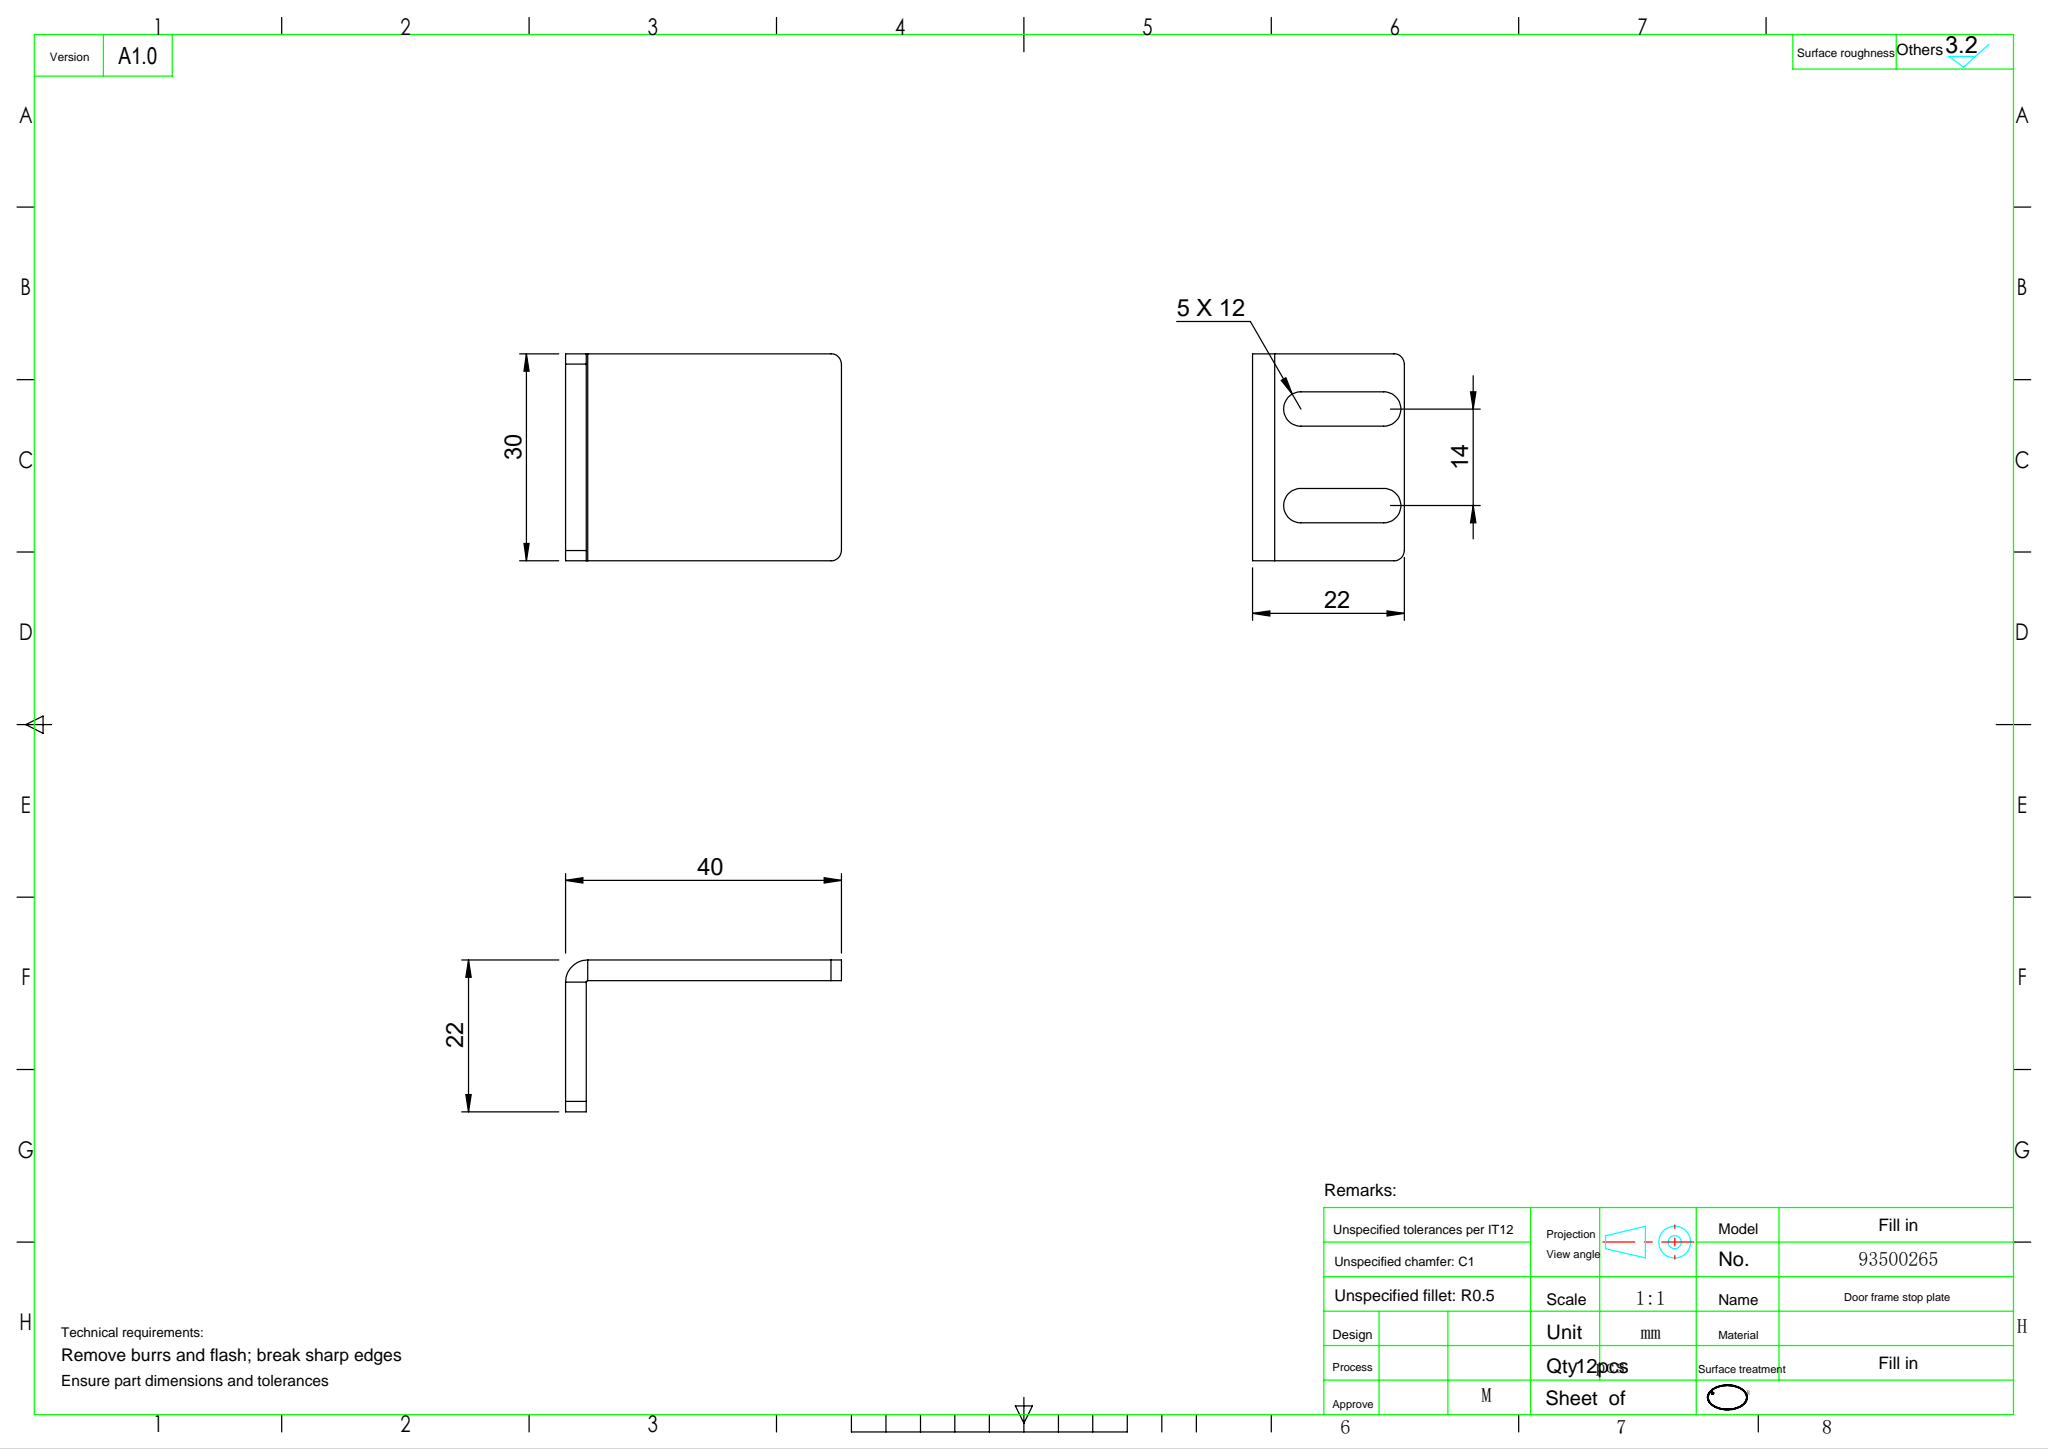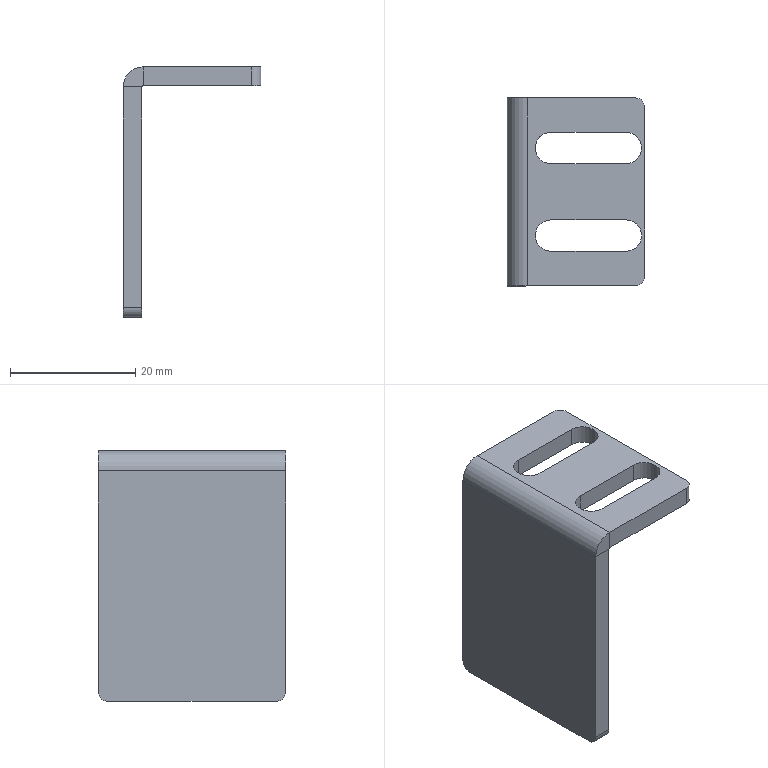Part | SolidWorks | features Fillet 1, FlatPattern 1, ICE 1, SMBaseFlange 1, SheetMetal 1 | 1 solid | 28 faces | box 22 x 30 x 40 mm | volume 4761 mm3 | plane 16 | cylinder 12 | commonest cylinder face diameters 5 x6 3 x4 0.4 x1 6.4 x1
STEP:
#1=CARTESIAN_POINT('',(4.5,8.,0.));
#2=VERTEX_POINT('',#1);
#3=CARTESIAN_POINT('',(7.,10.5,0.));
#4=VERTEX_POINT('',#3);
#5=CARTESIAN_POINT('',(7.,8.,0.));
#6=DIRECTION('',(0.,0.,-1.));
#7=DIRECTION('',(-1.,0.,0.));
#8=AXIS2_PLACEMENT_3D('',#5,#6,#7);
#9=CIRCLE('',#8,2.5);
#10=EDGE_CURVE('',#2,#4,#9,.T.);
#11=ORIENTED_EDGE('',*,*,#10,.F.);
#12=CARTESIAN_POINT('',(4.5,8.,-3.));
#13=VERTEX_POINT('',#12);
#14=CARTESIAN_POINT('',(4.5,8.,7.));
#15=DIRECTION('',(0.,0.,-1.));
#16=VECTOR('',#15,1000.);
#17=LINE('',#14,#16);
#18=EDGE_CURVE('',#2,#13,#17,.T.);
#19=ORIENTED_EDGE('',*,*,#18,.T.);
#20=CARTESIAN_POINT('',(7.,10.5,-3.));
#21=VERTEX_POINT('',#20);
#22=CARTESIAN_POINT('',(7.,8.,-3.));
#23=DIRECTION('',(0.,0.,-1.));
#24=DIRECTION('',(1.,0.,0.));
#25=AXIS2_PLACEMENT_3D('',#22,#23,#24);
#26=CIRCLE('',#25,2.5);
#27=EDGE_CURVE('',#13,#21,#26,.T.);
#28=ORIENTED_EDGE('',*,*,#27,.T.);
#29=CARTESIAN_POINT('',(7.,10.5,7.));
#30=DIRECTION('',(0.,0.,-1.));
#31=VECTOR('',#30,1000.);
#32=LINE('',#29,#31);
#33=EDGE_CURVE('',#4,#21,#32,.T.);
#34=ORIENTED_EDGE('',*,*,#33,.F.);
#35=EDGE_LOOP('',(#11,#19,#28,#34));
#36=FACE_OUTER_BOUND('',#35,.T.);
#37=CARTESIAN_POINT('',(7.,8.,7.));
#38=DIRECTION('',(0.,0.,-1.));
#39=DIRECTION('',(-1.,0.,0.));
#40=AXIS2_PLACEMENT_3D('',#37,#38,#39);
#41=CYLINDRICAL_SURFACE('',#40,2.5);
#42=ADVANCED_FACE('',(#36),#41,.F.);
#43=CARTESIAN_POINT('',(4.5,22.,0.));
#44=VERTEX_POINT('',#43);
#45=CARTESIAN_POINT('',(7.,24.5,0.));
#46=VERTEX_POINT('',#45);
#47=CARTESIAN_POINT('',(7.,22.,0.));
#48=DIRECTION('',(0.,0.,-1.));
#49=DIRECTION('',(-1.,0.,0.));
#50=AXIS2_PLACEMENT_3D('',#47,#48,#49);
#51=CIRCLE('',#50,2.5);
#52=EDGE_CURVE('',#44,#46,#51,.T.);
#53=ORIENTED_EDGE('',*,*,#52,.F.);
#54=CARTESIAN_POINT('',(4.5,22.,-3.));
#55=VERTEX_POINT('',#54);
#56=CARTESIAN_POINT('',(4.5,22.,7.));
#57=DIRECTION('',(0.,0.,-1.));
#58=VECTOR('',#57,1000.);
#59=LINE('',#56,#58);
#60=EDGE_CURVE('',#44,#55,#59,.T.);
#61=ORIENTED_EDGE('',*,*,#60,.T.);
#62=CARTESIAN_POINT('',(7.,24.5,-3.));
#63=VERTEX_POINT('',#62);
#64=CARTESIAN_POINT('',(7.,22.,-3.));
#65=DIRECTION('',(0.,0.,-1.));
#66=DIRECTION('',(-1.,0.,0.));
#67=AXIS2_PLACEMENT_3D('',#64,#65,#66);
#68=CIRCLE('',#67,2.5);
#69=EDGE_CURVE('',#55,#63,#68,.T.);
#70=ORIENTED_EDGE('',*,*,#69,.T.);
#71=CARTESIAN_POINT('',(7.,24.5,7.));
#72=DIRECTION('',(0.,0.,-1.));
#73=VECTOR('',#72,1000.);
#74=LINE('',#71,#73);
#75=EDGE_CURVE('',#46,#63,#74,.T.);
#76=ORIENTED_EDGE('',*,*,#75,.F.);
#77=EDGE_LOOP('',(#53,#61,#70,#76));
#78=FACE_OUTER_BOUND('',#77,.T.);
#79=CARTESIAN_POINT('',(7.,22.,7.));
#80=DIRECTION('',(0.,0.,-1.));
#81=DIRECTION('',(-1.,0.,0.));
#82=AXIS2_PLACEMENT_3D('',#79,#80,#81);
#83=CYLINDRICAL_SURFACE('',#82,2.5);
#84=ADVANCED_FACE('',(#78),#83,.F.);
#85=CARTESIAN_POINT('',(0.,30.,-3.2));
#86=VERTEX_POINT('',#85);
#87=CARTESIAN_POINT('',(3.,30.,-3.2));
#88=VERTEX_POINT('',#87);
#89=CARTESIAN_POINT('',(0.,30.,-3.2));
#90=DIRECTION('',(1.,0.,0.));
#91=VECTOR('',#90,1000.);
#92=LINE('',#89,#91);
#93=EDGE_CURVE('',#86,#88,#92,.T.);
#94=ORIENTED_EDGE('',*,*,#93,.F.);
#95=CARTESIAN_POINT('',(3.2,30.,0.));
#96=VERTEX_POINT('',#95);
#97=CARTESIAN_POINT('',(3.2,30.,-3.2));
#98=DIRECTION('',(0.,1.,0.));
#99=DIRECTION('',(0.,0.,-1.));
#100=AXIS2_PLACEMENT_3D('',#97,#98,#99);
#101=CIRCLE('',#100,3.2);
#102=EDGE_CURVE('',#86,#96,#101,.T.);
#103=ORIENTED_EDGE('',*,*,#102,.T.);
#104=CARTESIAN_POINT('',(3.2,30.,-3.));
#105=VERTEX_POINT('',#104);
#106=CARTESIAN_POINT('',(3.2,30.,-3.));
#107=DIRECTION('',(0.,0.,1.));
#108=VECTOR('',#107,1000.);
#109=LINE('',#106,#108);
#110=EDGE_CURVE('',#105,#96,#109,.T.);
#111=ORIENTED_EDGE('',*,*,#110,.F.);
#112=CARTESIAN_POINT('',(3.2,30.,-3.2));
#113=DIRECTION('',(0.,1.,0.));
#114=DIRECTION('',(1.,0.,0.));
#115=AXIS2_PLACEMENT_3D('',#112,#113,#114);
#116=CIRCLE('',#115,0.2);
#117=EDGE_CURVE('',#88,#105,#116,.T.);
#118=ORIENTED_EDGE('',*,*,#117,.F.);
#119=EDGE_LOOP('',(#94,#103,#111,#118));
#120=FACE_OUTER_BOUND('',#119,.T.);
#121=CARTESIAN_POINT('',(0.,30.,-3.2));
#122=DIRECTION('',(0.,1.,0.));
#123=DIRECTION('',(0.,0.,1.));
#124=AXIS2_PLACEMENT_3D('',#121,#122,#123);
#125=PLANE('',#124);
#126=ADVANCED_FACE('',(#120),#125,.T.);
#127=CARTESIAN_POINT('',(3.,30.,-38.5));
#128=VERTEX_POINT('',#127);
#129=CARTESIAN_POINT('',(3.,30.,-40.));
#130=DIRECTION('',(0.,0.,1.));
#131=VECTOR('',#130,1000.);
#132=LINE('',#129,#131);
#133=EDGE_CURVE('',#128,#88,#132,.T.);
#134=ORIENTED_EDGE('',*,*,#133,.F.);
#135=CARTESIAN_POINT('',(0.,30.,-38.5));
#136=VERTEX_POINT('',#135);
#137=CARTESIAN_POINT('',(3.2,30.,-38.5));
#138=DIRECTION('',(-1.,0.,0.));
#139=VECTOR('',#138,1000.);
#140=LINE('',#137,#139);
#141=EDGE_CURVE('',#128,#136,#140,.T.);
#142=ORIENTED_EDGE('',*,*,#141,.T.);
#143=CARTESIAN_POINT('',(0.,30.,-40.));
#144=DIRECTION('',(0.,0.,1.));
#145=VECTOR('',#144,1000.);
#146=LINE('',#143,#145);
#147=EDGE_CURVE('',#136,#86,#146,.T.);
#148=ORIENTED_EDGE('',*,*,#147,.T.);
#149=ORIENTED_EDGE('',*,*,#93,.T.);
#150=EDGE_LOOP('',(#134,#142,#148,#149));
#151=FACE_OUTER_BOUND('',#150,.T.);
#152=CARTESIAN_POINT('',(3.2,30.,-3.));
#153=DIRECTION('',(0.,1.,0.));
#154=DIRECTION('',(0.,0.,1.));
#155=AXIS2_PLACEMENT_3D('',#152,#153,#154);
#156=PLANE('',#155);
#157=ADVANCED_FACE('',(#151),#156,.T.);
#158=CARTESIAN_POINT('',(3.2,0.,0.));
#159=VERTEX_POINT('',#158);
#160=CARTESIAN_POINT('',(3.2,0.,-3.));
#161=VERTEX_POINT('',#160);
#162=CARTESIAN_POINT('',(3.2,0.,0.));
#163=DIRECTION('',(0.,0.,-1.));
#164=VECTOR('',#163,1000.);
#165=LINE('',#162,#164);
#166=EDGE_CURVE('',#159,#161,#165,.T.);
#167=ORIENTED_EDGE('',*,*,#166,.F.);
#168=CARTESIAN_POINT('',(0.,0.,-3.2));
#169=VERTEX_POINT('',#168);
#170=CARTESIAN_POINT('',(3.2,0.,-3.2));
#171=DIRECTION('',(0.,1.,0.));
#172=DIRECTION('',(0.,0.,-1.));
#173=AXIS2_PLACEMENT_3D('',#170,#171,#172);
#174=CIRCLE('',#173,3.2);
#175=EDGE_CURVE('',#169,#159,#174,.T.);
#176=ORIENTED_EDGE('',*,*,#175,.F.);
#177=CARTESIAN_POINT('',(3.,0.,-3.2));
#178=VERTEX_POINT('',#177);
#179=CARTESIAN_POINT('',(3.,0.,-3.2));
#180=DIRECTION('',(-1.,0.,0.));
#181=VECTOR('',#180,1000.);
#182=LINE('',#179,#181);
#183=EDGE_CURVE('',#178,#169,#182,.T.);
#184=ORIENTED_EDGE('',*,*,#183,.F.);
#185=CARTESIAN_POINT('',(3.2,0.,-3.2));
#186=DIRECTION('',(0.,1.,0.));
#187=DIRECTION('',(1.,0.,0.));
#188=AXIS2_PLACEMENT_3D('',#185,#186,#187);
#189=CIRCLE('',#188,0.2);
#190=EDGE_CURVE('',#178,#161,#189,.T.);
#191=ORIENTED_EDGE('',*,*,#190,.T.);
#192=EDGE_LOOP('',(#167,#176,#184,#191));
#193=FACE_OUTER_BOUND('',#192,.T.);
#194=CARTESIAN_POINT('',(3.2,0.,0.));
#195=DIRECTION('',(0.,-1.,0.));
#196=DIRECTION('',(0.,0.,-1.));
#197=AXIS2_PLACEMENT_3D('',#194,#195,#196);
#198=PLANE('',#197);
#199=ADVANCED_FACE('',(#193),#198,.T.);
#200=CARTESIAN_POINT('',(20.5,0.,-3.));
#201=VERTEX_POINT('',#200);
#202=CARTESIAN_POINT('',(0.,0.,-3.));
#203=DIRECTION('',(1.,0.,0.));
#204=VECTOR('',#203,1000.);
#205=LINE('',#202,#204);
#206=EDGE_CURVE('',#161,#201,#205,.T.);
#207=ORIENTED_EDGE('',*,*,#206,.T.);
#208=CARTESIAN_POINT('',(20.5,0.,0.));
#209=VERTEX_POINT('',#208);
#210=CARTESIAN_POINT('',(20.5,0.,-3.2));
#211=DIRECTION('',(0.,0.,1.));
#212=VECTOR('',#211,1000.);
#213=LINE('',#210,#212);
#214=EDGE_CURVE('',#201,#209,#213,.T.);
#215=ORIENTED_EDGE('',*,*,#214,.T.);
#216=CARTESIAN_POINT('',(0.,0.,0.));
#217=DIRECTION('',(1.,0.,0.));
#218=VECTOR('',#217,1000.);
#219=LINE('',#216,#218);
#220=EDGE_CURVE('',#159,#209,#219,.T.);
#221=ORIENTED_EDGE('',*,*,#220,.F.);
#222=ORIENTED_EDGE('',*,*,#166,.T.);
#223=EDGE_LOOP('',(#207,#215,#221,#222));
#224=FACE_OUTER_BOUND('',#223,.T.);
#225=CARTESIAN_POINT('',(3.,0.,-3.2));
#226=DIRECTION('',(0.,-1.,0.));
#227=DIRECTION('',(0.,0.,-1.));
#228=AXIS2_PLACEMENT_3D('',#225,#226,#227);
#229=PLANE('',#228);
#230=ADVANCED_FACE('',(#224),#229,.T.);
#231=CARTESIAN_POINT('',(19.,10.5,0.));
#232=VERTEX_POINT('',#231);
#233=CARTESIAN_POINT('',(0.,10.5,0.));
#234=DIRECTION('',(1.,0.,0.));
#235=VECTOR('',#234,1000.);
#236=LINE('',#233,#235);
#237=EDGE_CURVE('',#4,#232,#236,.T.);
#238=ORIENTED_EDGE('',*,*,#237,.T.);
#239=CARTESIAN_POINT('',(19.,5.5,0.));
#240=VERTEX_POINT('',#239);
#241=CARTESIAN_POINT('',(19.,8.,0.));
#242=DIRECTION('',(0.,0.,-1.));
#243=DIRECTION('',(-1.,0.,0.));
#244=AXIS2_PLACEMENT_3D('',#241,#242,#243);
#245=CIRCLE('',#244,2.5);
#246=EDGE_CURVE('',#232,#240,#245,.T.);
#247=ORIENTED_EDGE('',*,*,#246,.T.);
#248=CARTESIAN_POINT('',(7.,5.5,0.));
#249=VERTEX_POINT('',#248);
#250=CARTESIAN_POINT('',(0.,5.5,0.));
#251=DIRECTION('',(-1.,0.,0.));
#252=VECTOR('',#251,1000.);
#253=LINE('',#250,#252);
#254=EDGE_CURVE('',#240,#249,#253,.T.);
#255=ORIENTED_EDGE('',*,*,#254,.T.);
#256=CARTESIAN_POINT('',(7.,8.,0.));
#257=DIRECTION('',(0.,0.,-1.));
#258=DIRECTION('',(-1.,0.,0.));
#259=AXIS2_PLACEMENT_3D('',#256,#257,#258);
#260=CIRCLE('',#259,2.5);
#261=EDGE_CURVE('',#249,#2,#260,.T.);
#262=ORIENTED_EDGE('',*,*,#261,.T.);
#263=ORIENTED_EDGE('',*,*,#10,.T.);
#264=EDGE_LOOP('',(#238,#247,#255,#262,#263));
#265=FACE_BOUND('',#264,.T.);
#266=CARTESIAN_POINT('',(19.,24.5,0.));
#267=VERTEX_POINT('',#266);
#268=CARTESIAN_POINT('',(0.,24.5,0.));
#269=DIRECTION('',(1.,0.,0.));
#270=VECTOR('',#269,1000.);
#271=LINE('',#268,#270);
#272=EDGE_CURVE('',#46,#267,#271,.T.);
#273=ORIENTED_EDGE('',*,*,#272,.T.);
#274=CARTESIAN_POINT('',(19.,19.5,0.));
#275=VERTEX_POINT('',#274);
#276=CARTESIAN_POINT('',(19.,22.,0.));
#277=DIRECTION('',(0.,0.,-1.));
#278=DIRECTION('',(-1.,0.,0.));
#279=AXIS2_PLACEMENT_3D('',#276,#277,#278);
#280=CIRCLE('',#279,2.5);
#281=EDGE_CURVE('',#267,#275,#280,.T.);
#282=ORIENTED_EDGE('',*,*,#281,.T.);
#283=CARTESIAN_POINT('',(7.,19.5,0.));
#284=VERTEX_POINT('',#283);
#285=CARTESIAN_POINT('',(0.,19.5,0.));
#286=DIRECTION('',(-1.,0.,0.));
#287=VECTOR('',#286,1000.);
#288=LINE('',#285,#287);
#289=EDGE_CURVE('',#275,#284,#288,.T.);
#290=ORIENTED_EDGE('',*,*,#289,.T.);
#291=CARTESIAN_POINT('',(7.,22.,0.));
#292=DIRECTION('',(0.,0.,-1.));
#293=DIRECTION('',(-1.,0.,0.));
#294=AXIS2_PLACEMENT_3D('',#291,#292,#293);
#295=CIRCLE('',#294,2.5);
#296=EDGE_CURVE('',#284,#44,#295,.T.);
#297=ORIENTED_EDGE('',*,*,#296,.T.);
#298=ORIENTED_EDGE('',*,*,#52,.T.);
#299=EDGE_LOOP('',(#273,#282,#290,#297,#298));
#300=FACE_BOUND('',#299,.T.);
#301=CARTESIAN_POINT('',(22.,28.5,0.));
#302=VERTEX_POINT('',#301);
#303=CARTESIAN_POINT('',(22.,1.5,0.));
#304=VERTEX_POINT('',#303);
#305=CARTESIAN_POINT('',(22.,30.,0.));
#306=DIRECTION('',(0.,-1.,0.));
#307=VECTOR('',#306,1000.);
#308=LINE('',#305,#307);
#309=EDGE_CURVE('',#302,#304,#308,.T.);
#310=ORIENTED_EDGE('',*,*,#309,.F.);
#311=CARTESIAN_POINT('',(20.5,30.,0.));
#312=VERTEX_POINT('',#311);
#313=CARTESIAN_POINT('',(20.5,28.5,0.));
#314=DIRECTION('',(0.,0.,1.));
#315=DIRECTION('',(-1.,0.,0.));
#316=AXIS2_PLACEMENT_3D('',#313,#314,#315);
#317=CIRCLE('',#316,1.5);
#318=EDGE_CURVE('',#302,#312,#317,.T.);
#319=ORIENTED_EDGE('',*,*,#318,.T.);
#320=CARTESIAN_POINT('',(0.,30.,0.));
#321=DIRECTION('',(1.,0.,0.));
#322=VECTOR('',#321,1000.);
#323=LINE('',#320,#322);
#324=EDGE_CURVE('',#96,#312,#323,.T.);
#325=ORIENTED_EDGE('',*,*,#324,.F.);
#326=CARTESIAN_POINT('',(3.2,30.,0.));
#327=DIRECTION('',(0.,-1.,0.));
#328=VECTOR('',#327,1000.);
#329=LINE('',#326,#328);
#330=EDGE_CURVE('',#96,#159,#329,.T.);
#331=ORIENTED_EDGE('',*,*,#330,.T.);
#332=ORIENTED_EDGE('',*,*,#220,.T.);
#333=CARTESIAN_POINT('',(20.5,1.5,0.));
#334=DIRECTION('',(0.,0.,1.));
#335=DIRECTION('',(-1.,0.,0.));
#336=AXIS2_PLACEMENT_3D('',#333,#334,#335);
#337=CIRCLE('',#336,1.5);
#338=EDGE_CURVE('',#209,#304,#337,.T.);
#339=ORIENTED_EDGE('',*,*,#338,.T.);
#340=EDGE_LOOP('',(#310,#319,#325,#331,#332,#339));
#341=FACE_OUTER_BOUND('',#340,.T.);
#342=CARTESIAN_POINT('',(0.,30.,0.));
#343=DIRECTION('',(0.,0.,-1.));
#344=DIRECTION('',(-1.,0.,0.));
#345=AXIS2_PLACEMENT_3D('',#342,#343,#344);
#346=PLANE('',#345);
#347=ADVANCED_FACE('',(#265,#300,#341),#346,.F.);
#348=CARTESIAN_POINT('',(22.,28.5,-3.));
#349=VERTEX_POINT('',#348);
#350=CARTESIAN_POINT('',(22.,1.5,-3.));
#351=VERTEX_POINT('',#350);
#352=CARTESIAN_POINT('',(22.,30.,-3.));
#353=DIRECTION('',(0.,-1.,0.));
#354=VECTOR('',#353,1000.);
#355=LINE('',#352,#354);
#356=EDGE_CURVE('',#349,#351,#355,.T.);
#357=ORIENTED_EDGE('',*,*,#356,.F.);
#358=CARTESIAN_POINT('',(22.,28.5,-3.));
#359=DIRECTION('',(0.,0.,1.));
#360=VECTOR('',#359,1000.);
#361=LINE('',#358,#360);
#362=EDGE_CURVE('',#349,#302,#361,.T.);
#363=ORIENTED_EDGE('',*,*,#362,.T.);
#364=ORIENTED_EDGE('',*,*,#309,.T.);
#365=CARTESIAN_POINT('',(22.,1.5,-3.));
#366=DIRECTION('',(0.,0.,-1.));
#367=VECTOR('',#366,1000.);
#368=LINE('',#365,#367);
#369=EDGE_CURVE('',#304,#351,#368,.T.);
#370=ORIENTED_EDGE('',*,*,#369,.T.);
#371=EDGE_LOOP('',(#357,#363,#364,#370));
#372=FACE_OUTER_BOUND('',#371,.T.);
#373=CARTESIAN_POINT('',(22.,30.,-3.));
#374=DIRECTION('',(1.,0.,0.));
#375=DIRECTION('',(0.,0.,-1.));
#376=AXIS2_PLACEMENT_3D('',#373,#374,#375);
#377=PLANE('',#376);
#378=ADVANCED_FACE('',(#372),#377,.T.);
#379=CARTESIAN_POINT('',(19.,10.5,-3.));
#380=VERTEX_POINT('',#379);
#381=CARTESIAN_POINT('',(19.,5.5,-3.));
#382=VERTEX_POINT('',#381);
#383=CARTESIAN_POINT('',(19.,8.,-3.));
#384=DIRECTION('',(0.,0.,-1.));
#385=DIRECTION('',(1.,0.,0.));
#386=AXIS2_PLACEMENT_3D('',#383,#384,#385);
#387=CIRCLE('',#386,2.5);
#388=EDGE_CURVE('',#380,#382,#387,.T.);
#389=ORIENTED_EDGE('',*,*,#388,.F.);
#390=CARTESIAN_POINT('',(19.,10.5,-3.));
#391=DIRECTION('',(1.,0.,0.));
#392=VECTOR('',#391,1000.);
#393=LINE('',#390,#392);
#394=EDGE_CURVE('',#21,#380,#393,.T.);
#395=ORIENTED_EDGE('',*,*,#394,.F.);
#396=ORIENTED_EDGE('',*,*,#27,.F.);
#397=CARTESIAN_POINT('',(7.,5.5,-3.));
#398=VERTEX_POINT('',#397);
#399=CARTESIAN_POINT('',(7.,8.,-3.));
#400=DIRECTION('',(0.,0.,-1.));
#401=DIRECTION('',(1.,0.,0.));
#402=AXIS2_PLACEMENT_3D('',#399,#400,#401);
#403=CIRCLE('',#402,2.5);
#404=EDGE_CURVE('',#398,#13,#403,.T.);
#405=ORIENTED_EDGE('',*,*,#404,.F.);
#406=CARTESIAN_POINT('',(19.,5.5,-3.));
#407=DIRECTION('',(-1.,0.,0.));
#408=VECTOR('',#407,1000.);
#409=LINE('',#406,#408);
#410=EDGE_CURVE('',#382,#398,#409,.T.);
#411=ORIENTED_EDGE('',*,*,#410,.F.);
#412=EDGE_LOOP('',(#389,#395,#396,#405,#411));
#413=FACE_BOUND('',#412,.T.);
#414=CARTESIAN_POINT('',(19.,24.5,-3.));
#415=VERTEX_POINT('',#414);
#416=CARTESIAN_POINT('',(19.,19.5,-3.));
#417=VERTEX_POINT('',#416);
#418=CARTESIAN_POINT('',(19.,22.,-3.));
#419=DIRECTION('',(0.,0.,-1.));
#420=DIRECTION('',(-1.,0.,0.));
#421=AXIS2_PLACEMENT_3D('',#418,#419,#420);
#422=CIRCLE('',#421,2.5);
#423=EDGE_CURVE('',#415,#417,#422,.T.);
#424=ORIENTED_EDGE('',*,*,#423,.F.);
#425=CARTESIAN_POINT('',(19.,24.5,-3.));
#426=DIRECTION('',(1.,0.,0.));
#427=VECTOR('',#426,1000.);
#428=LINE('',#425,#427);
#429=EDGE_CURVE('',#63,#415,#428,.T.);
#430=ORIENTED_EDGE('',*,*,#429,.F.);
#431=ORIENTED_EDGE('',*,*,#69,.F.);
#432=CARTESIAN_POINT('',(7.,19.5,-3.));
#433=VERTEX_POINT('',#432);
#434=CARTESIAN_POINT('',(7.,22.,-3.));
#435=DIRECTION('',(0.,0.,-1.));
#436=DIRECTION('',(-1.,0.,0.));
#437=AXIS2_PLACEMENT_3D('',#434,#435,#436);
#438=CIRCLE('',#437,2.5);
#439=EDGE_CURVE('',#433,#55,#438,.T.);
#440=ORIENTED_EDGE('',*,*,#439,.F.);
#441=CARTESIAN_POINT('',(19.,19.5,-3.));
#442=DIRECTION('',(-1.,0.,0.));
#443=VECTOR('',#442,1000.);
#444=LINE('',#441,#443);
#445=EDGE_CURVE('',#417,#433,#444,.T.);
#446=ORIENTED_EDGE('',*,*,#445,.F.);
#447=EDGE_LOOP('',(#424,#430,#431,#440,#446));
#448=FACE_BOUND('',#447,.T.);
#449=CARTESIAN_POINT('',(20.5,30.,-3.));
#450=VERTEX_POINT('',#449);
#451=CARTESIAN_POINT('',(0.,30.,-3.));
#452=DIRECTION('',(1.,0.,0.));
#453=VECTOR('',#452,1000.);
#454=LINE('',#451,#453);
#455=EDGE_CURVE('',#105,#450,#454,.T.);
#456=ORIENTED_EDGE('',*,*,#455,.T.);
#457=CARTESIAN_POINT('',(20.5,28.5,-3.));
#458=DIRECTION('',(0.,0.,-1.));
#459=DIRECTION('',(-1.,0.,0.));
#460=AXIS2_PLACEMENT_3D('',#457,#458,#459);
#461=CIRCLE('',#460,1.5);
#462=EDGE_CURVE('',#450,#349,#461,.T.);
#463=ORIENTED_EDGE('',*,*,#462,.T.);
#464=ORIENTED_EDGE('',*,*,#356,.T.);
#465=CARTESIAN_POINT('',(20.5,1.5,-3.));
#466=DIRECTION('',(0.,0.,-1.));
#467=DIRECTION('',(-1.,0.,0.));
#468=AXIS2_PLACEMENT_3D('',#465,#466,#467);
#469=CIRCLE('',#468,1.5);
#470=EDGE_CURVE('',#351,#201,#469,.T.);
#471=ORIENTED_EDGE('',*,*,#470,.T.);
#472=ORIENTED_EDGE('',*,*,#206,.F.);
#473=CARTESIAN_POINT('',(3.2,30.,-3.));
#474=DIRECTION('',(0.,-1.,0.));
#475=VECTOR('',#474,1000.);
#476=LINE('',#473,#475);
#477=EDGE_CURVE('',#105,#161,#476,.T.);
#478=ORIENTED_EDGE('',*,*,#477,.F.);
#479=EDGE_LOOP('',(#456,#463,#464,#471,#472,#478));
#480=FACE_OUTER_BOUND('',#479,.T.);
#481=CARTESIAN_POINT('',(0.,30.,-3.));
#482=DIRECTION('',(0.,0.,-1.));
#483=DIRECTION('',(-1.,0.,0.));
#484=AXIS2_PLACEMENT_3D('',#481,#482,#483);
#485=PLANE('',#484);
#486=ADVANCED_FACE('',(#413,#448,#480),#485,.T.);
#487=ORIENTED_EDGE('',*,*,#190,.F.);
#488=CARTESIAN_POINT('',(3.,30.,-3.2));
#489=DIRECTION('',(0.,-1.,0.));
#490=VECTOR('',#489,1000.);
#491=LINE('',#488,#490);
#492=EDGE_CURVE('',#88,#178,#491,.T.);
#493=ORIENTED_EDGE('',*,*,#492,.F.);
#494=ORIENTED_EDGE('',*,*,#117,.T.);
#495=ORIENTED_EDGE('',*,*,#477,.T.);
#496=EDGE_LOOP('',(#487,#493,#494,#495));
#497=FACE_OUTER_BOUND('',#496,.T.);
#498=CARTESIAN_POINT('',(3.2,30.,-3.2));
#499=DIRECTION('',(0.,-1.,0.));
#500=DIRECTION('',(0.,0.,-1.));
#501=AXIS2_PLACEMENT_3D('',#498,#499,#500);
#502=CYLINDRICAL_SURFACE('',#501,0.2);
#503=ADVANCED_FACE('',(#497),#502,.F.);
#504=CARTESIAN_POINT('',(3.,28.5,-40.));
#505=VERTEX_POINT('',#504);
#506=CARTESIAN_POINT('',(3.,1.5,-40.));
#507=VERTEX_POINT('',#506);
#508=CARTESIAN_POINT('',(3.,30.,-40.));
#509=DIRECTION('',(0.,-1.,0.));
#510=VECTOR('',#509,1000.);
#511=LINE('',#508,#510);
#512=EDGE_CURVE('',#505,#507,#511,.T.);
#513=ORIENTED_EDGE('',*,*,#512,.F.);
#514=CARTESIAN_POINT('',(3.,28.5,-38.5));
#515=DIRECTION('',(1.,0.,0.));
#516=DIRECTION('',(0.,0.,-1.));
#517=AXIS2_PLACEMENT_3D('',#514,#515,#516);
#518=CIRCLE('',#517,1.5);
#519=EDGE_CURVE('',#505,#128,#518,.T.);
#520=ORIENTED_EDGE('',*,*,#519,.T.);
#521=ORIENTED_EDGE('',*,*,#133,.T.);
#522=ORIENTED_EDGE('',*,*,#492,.T.);
#523=CARTESIAN_POINT('',(3.,0.,-38.5));
#524=VERTEX_POINT('',#523);
#525=CARTESIAN_POINT('',(3.,0.,-40.));
#526=DIRECTION('',(0.,0.,1.));
#527=VECTOR('',#526,1000.);
#528=LINE('',#525,#527);
#529=EDGE_CURVE('',#524,#178,#528,.T.);
#530=ORIENTED_EDGE('',*,*,#529,.F.);
#531=CARTESIAN_POINT('',(3.,1.5,-38.5));
#532=DIRECTION('',(1.,0.,0.));
#533=DIRECTION('',(0.,0.,-1.));
#534=AXIS2_PLACEMENT_3D('',#531,#532,#533);
#535=CIRCLE('',#534,1.5);
#536=EDGE_CURVE('',#524,#507,#535,.T.);
#537=ORIENTED_EDGE('',*,*,#536,.T.);
#538=EDGE_LOOP('',(#513,#520,#521,#522,#530,#537));
#539=FACE_OUTER_BOUND('',#538,.T.);
#540=CARTESIAN_POINT('',(3.,30.,-40.));
#541=DIRECTION('',(1.,0.,0.));
#542=DIRECTION('',(0.,0.,-1.));
#543=AXIS2_PLACEMENT_3D('',#540,#541,#542);
#544=PLANE('',#543);
#545=ADVANCED_FACE('',(#539),#544,.T.);
#546=CARTESIAN_POINT('',(0.,28.5,-40.));
#547=VERTEX_POINT('',#546);
#548=CARTESIAN_POINT('',(0.,1.5,-40.));
#549=VERTEX_POINT('',#548);
#550=CARTESIAN_POINT('',(0.,30.,-40.));
#551=DIRECTION('',(0.,-1.,0.));
#552=VECTOR('',#551,1000.);
#553=LINE('',#550,#552);
#554=EDGE_CURVE('',#547,#549,#553,.T.);
#555=ORIENTED_EDGE('',*,*,#554,.F.);
#556=CARTESIAN_POINT('',(0.,28.5,-40.));
#557=DIRECTION('',(1.,0.,0.));
#558=VECTOR('',#557,1000.);
#559=LINE('',#556,#558);
#560=EDGE_CURVE('',#547,#505,#559,.T.);
#561=ORIENTED_EDGE('',*,*,#560,.T.);
#562=ORIENTED_EDGE('',*,*,#512,.T.);
#563=CARTESIAN_POINT('',(0.,1.5,-40.));
#564=DIRECTION('',(-1.,0.,0.));
#565=VECTOR('',#564,1000.);
#566=LINE('',#563,#565);
#567=EDGE_CURVE('',#507,#549,#566,.T.);
#568=ORIENTED_EDGE('',*,*,#567,.T.);
#569=EDGE_LOOP('',(#555,#561,#562,#568));
#570=FACE_OUTER_BOUND('',#569,.T.);
#571=CARTESIAN_POINT('',(0.,30.,-40.));
#572=DIRECTION('',(0.,0.,-1.));
#573=DIRECTION('',(-1.,0.,0.));
#574=AXIS2_PLACEMENT_3D('',#571,#572,#573);
#575=PLANE('',#574);
#576=ADVANCED_FACE('',(#570),#575,.T.);
#577=ORIENTED_EDGE('',*,*,#147,.F.);
#578=CARTESIAN_POINT('',(0.,28.5,-38.5));
#579=DIRECTION('',(-1.,0.,0.));
#580=DIRECTION('',(0.,0.,-1.));
#581=AXIS2_PLACEMENT_3D('',#578,#579,#580);
#582=CIRCLE('',#581,1.5);
#583=EDGE_CURVE('',#136,#547,#582,.T.);
#584=ORIENTED_EDGE('',*,*,#583,.T.);
#585=ORIENTED_EDGE('',*,*,#554,.T.);
#586=CARTESIAN_POINT('',(0.,0.,-38.5));
#587=VERTEX_POINT('',#586);
#588=CARTESIAN_POINT('',(0.,1.5,-38.5));
#589=DIRECTION('',(-1.,0.,0.));
#590=DIRECTION('',(0.,0.,-1.));
#591=AXIS2_PLACEMENT_3D('',#588,#589,#590);
#592=CIRCLE('',#591,1.5);
#593=EDGE_CURVE('',#549,#587,#592,.T.);
#594=ORIENTED_EDGE('',*,*,#593,.T.);
#595=CARTESIAN_POINT('',(0.,0.,-40.));
#596=DIRECTION('',(0.,0.,1.));
#597=VECTOR('',#596,1000.);
#598=LINE('',#595,#597);
#599=EDGE_CURVE('',#587,#169,#598,.T.);
#600=ORIENTED_EDGE('',*,*,#599,.T.);
#601=CARTESIAN_POINT('',(0.,30.,-3.2));
#602=DIRECTION('',(0.,-1.,0.));
#603=VECTOR('',#602,1000.);
#604=LINE('',#601,#603);
#605=EDGE_CURVE('',#86,#169,#604,.T.);
#606=ORIENTED_EDGE('',*,*,#605,.F.);
#607=EDGE_LOOP('',(#577,#584,#585,#594,#600,#606));
#608=FACE_OUTER_BOUND('',#607,.T.);
#609=CARTESIAN_POINT('',(0.,30.,-40.));
#610=DIRECTION('',(1.,0.,0.));
#611=DIRECTION('',(0.,0.,-1.));
#612=AXIS2_PLACEMENT_3D('',#609,#610,#611);
#613=PLANE('',#612);
#614=ADVANCED_FACE('',(#608),#613,.F.);
#615=ORIENTED_EDGE('',*,*,#175,.T.);
#616=ORIENTED_EDGE('',*,*,#330,.F.);
#617=ORIENTED_EDGE('',*,*,#102,.F.);
#618=ORIENTED_EDGE('',*,*,#605,.T.);
#619=EDGE_LOOP('',(#615,#616,#617,#618));
#620=FACE_OUTER_BOUND('',#619,.T.);
#621=CARTESIAN_POINT('',(3.2,30.,-3.2));
#622=DIRECTION('',(0.,-1.,0.));
#623=DIRECTION('',(0.,0.,-1.));
#624=AXIS2_PLACEMENT_3D('',#621,#622,#623);
#625=CYLINDRICAL_SURFACE('',#624,3.2);
#626=ADVANCED_FACE('',(#620),#625,.T.);
#627=ORIENTED_EDGE('',*,*,#324,.T.);
#628=CARTESIAN_POINT('',(20.5,30.,-3.2));
#629=DIRECTION('',(0.,0.,-1.));
#630=VECTOR('',#629,1000.);
#631=LINE('',#628,#630);
#632=EDGE_CURVE('',#312,#450,#631,.T.);
#633=ORIENTED_EDGE('',*,*,#632,.T.);
#634=ORIENTED_EDGE('',*,*,#455,.F.);
#635=ORIENTED_EDGE('',*,*,#110,.T.);
#636=EDGE_LOOP('',(#627,#633,#634,#635));
#637=FACE_OUTER_BOUND('',#636,.T.);
#638=CARTESIAN_POINT('',(3.2,30.,-3.2));
#639=DIRECTION('',(0.,1.,0.));
#640=DIRECTION('',(1.,0.,0.));
#641=AXIS2_PLACEMENT_3D('',#638,#639,#640);
#642=PLANE('',#641);
#643=ADVANCED_FACE('',(#637),#642,.T.);
#644=ORIENTED_EDGE('',*,*,#599,.F.);
#645=CARTESIAN_POINT('',(3.,0.,-38.5));
#646=DIRECTION('',(1.,0.,0.));
#647=VECTOR('',#646,1000.);
#648=LINE('',#645,#647);
#649=EDGE_CURVE('',#587,#524,#648,.T.);
#650=ORIENTED_EDGE('',*,*,#649,.T.);
#651=ORIENTED_EDGE('',*,*,#529,.T.);
#652=ORIENTED_EDGE('',*,*,#183,.T.);
#653=EDGE_LOOP('',(#644,#650,#651,#652));
#654=FACE_OUTER_BOUND('',#653,.T.);
#655=CARTESIAN_POINT('',(3.2,0.,-3.2));
#656=DIRECTION('',(0.,1.,0.));
#657=DIRECTION('',(1.,0.,0.));
#658=AXIS2_PLACEMENT_3D('',#655,#656,#657);
#659=PLANE('',#658);
#660=ADVANCED_FACE('',(#654),#659,.F.);
#661=ORIENTED_EDGE('',*,*,#583,.F.);
#662=ORIENTED_EDGE('',*,*,#141,.F.);
#663=ORIENTED_EDGE('',*,*,#519,.F.);
#664=ORIENTED_EDGE('',*,*,#560,.F.);
#665=EDGE_LOOP('',(#661,#662,#663,#664));
#666=FACE_OUTER_BOUND('',#665,.T.);
#667=CARTESIAN_POINT('',(0.,28.5,-38.5));
#668=DIRECTION('',(1.,0.,0.));
#669=DIRECTION('',(0.,0.,-1.));
#670=AXIS2_PLACEMENT_3D('',#667,#668,#669);
#671=CYLINDRICAL_SURFACE('',#670,1.5);
#672=ADVANCED_FACE('',(#666),#671,.T.);
#673=ORIENTED_EDGE('',*,*,#593,.F.);
#674=ORIENTED_EDGE('',*,*,#567,.F.);
#675=ORIENTED_EDGE('',*,*,#536,.F.);
#676=ORIENTED_EDGE('',*,*,#649,.F.);
#677=EDGE_LOOP('',(#673,#674,#675,#676));
#678=FACE_OUTER_BOUND('',#677,.T.);
#679=CARTESIAN_POINT('',(3.2,1.5,-38.5));
#680=DIRECTION('',(-1.,0.,0.));
#681=DIRECTION('',(0.,0.,1.));
#682=AXIS2_PLACEMENT_3D('',#679,#680,#681);
#683=CYLINDRICAL_SURFACE('',#682,1.5);
#684=ADVANCED_FACE('',(#678),#683,.T.);
#685=ORIENTED_EDGE('',*,*,#462,.F.);
#686=ORIENTED_EDGE('',*,*,#632,.F.);
#687=ORIENTED_EDGE('',*,*,#318,.F.);
#688=ORIENTED_EDGE('',*,*,#362,.F.);
#689=EDGE_LOOP('',(#685,#686,#687,#688));
#690=FACE_OUTER_BOUND('',#689,.T.);
#691=CARTESIAN_POINT('',(20.5,28.5,-3.));
#692=DIRECTION('',(0.,0.,1.));
#693=DIRECTION('',(1.,0.,0.));
#694=AXIS2_PLACEMENT_3D('',#691,#692,#693);
#695=CYLINDRICAL_SURFACE('',#694,1.5);
#696=ADVANCED_FACE('',(#690),#695,.T.);
#697=ORIENTED_EDGE('',*,*,#470,.F.);
#698=ORIENTED_EDGE('',*,*,#369,.F.);
#699=ORIENTED_EDGE('',*,*,#338,.F.);
#700=ORIENTED_EDGE('',*,*,#214,.F.);
#701=EDGE_LOOP('',(#697,#698,#699,#700));
#702=FACE_OUTER_BOUND('',#701,.T.);
#703=CARTESIAN_POINT('',(20.5,1.5,-3.2));
#704=DIRECTION('',(0.,0.,1.));
#705=DIRECTION('',(1.,0.,0.));
#706=AXIS2_PLACEMENT_3D('',#703,#704,#705);
#707=CYLINDRICAL_SURFACE('',#706,1.5);
#708=ADVANCED_FACE('',(#702),#707,.T.);
#709=CARTESIAN_POINT('',(19.,24.5,7.));
#710=DIRECTION('',(0.,0.,-1.));
#711=VECTOR('',#710,1000.);
#712=LINE('',#709,#711);
#713=EDGE_CURVE('',#267,#415,#712,.T.);
#714=ORIENTED_EDGE('',*,*,#713,.T.);
#715=ORIENTED_EDGE('',*,*,#423,.T.);
#716=CARTESIAN_POINT('',(19.,19.5,7.));
#717=DIRECTION('',(0.,0.,-1.));
#718=VECTOR('',#717,1000.);
#719=LINE('',#716,#718);
#720=EDGE_CURVE('',#275,#417,#719,.T.);
#721=ORIENTED_EDGE('',*,*,#720,.F.);
#722=ORIENTED_EDGE('',*,*,#281,.F.);
#723=EDGE_LOOP('',(#714,#715,#721,#722));
#724=FACE_OUTER_BOUND('',#723,.T.);
#725=CARTESIAN_POINT('',(19.,22.,7.));
#726=DIRECTION('',(0.,0.,-1.));
#727=DIRECTION('',(-1.,0.,0.));
#728=AXIS2_PLACEMENT_3D('',#725,#726,#727);
#729=CYLINDRICAL_SURFACE('',#728,2.5);
#730=ADVANCED_FACE('',(#724),#729,.F.);
#731=ORIENTED_EDGE('',*,*,#75,.T.);
#732=ORIENTED_EDGE('',*,*,#429,.T.);
#733=ORIENTED_EDGE('',*,*,#713,.F.);
#734=ORIENTED_EDGE('',*,*,#272,.F.);
#735=EDGE_LOOP('',(#731,#732,#733,#734));
#736=FACE_OUTER_BOUND('',#735,.T.);
#737=CARTESIAN_POINT('',(19.,24.5,7.));
#738=DIRECTION('',(0.,1.,0.));
#739=DIRECTION('',(0.,0.,1.));
#740=AXIS2_PLACEMENT_3D('',#737,#738,#739);
#741=PLANE('',#740);
#742=ADVANCED_FACE('',(#736),#741,.F.);
#743=ORIENTED_EDGE('',*,*,#60,.F.);
#744=ORIENTED_EDGE('',*,*,#296,.F.);
#745=CARTESIAN_POINT('',(7.,19.5,7.));
#746=DIRECTION('',(0.,0.,-1.));
#747=VECTOR('',#746,1000.);
#748=LINE('',#745,#747);
#749=EDGE_CURVE('',#284,#433,#748,.T.);
#750=ORIENTED_EDGE('',*,*,#749,.T.);
#751=ORIENTED_EDGE('',*,*,#439,.T.);
#752=EDGE_LOOP('',(#743,#744,#750,#751));
#753=FACE_OUTER_BOUND('',#752,.T.);
#754=CARTESIAN_POINT('',(7.,22.,7.));
#755=DIRECTION('',(0.,0.,-1.));
#756=DIRECTION('',(-1.,0.,0.));
#757=AXIS2_PLACEMENT_3D('',#754,#755,#756);
#758=CYLINDRICAL_SURFACE('',#757,2.5);
#759=ADVANCED_FACE('',(#753),#758,.F.);
#760=ORIENTED_EDGE('',*,*,#720,.T.);
#761=ORIENTED_EDGE('',*,*,#445,.T.);
#762=ORIENTED_EDGE('',*,*,#749,.F.);
#763=ORIENTED_EDGE('',*,*,#289,.F.);
#764=EDGE_LOOP('',(#760,#761,#762,#763));
#765=FACE_OUTER_BOUND('',#764,.T.);
#766=CARTESIAN_POINT('',(19.,19.5,7.));
#767=DIRECTION('',(0.,-1.,0.));
#768=DIRECTION('',(0.,0.,-1.));
#769=AXIS2_PLACEMENT_3D('',#766,#767,#768);
#770=PLANE('',#769);
#771=ADVANCED_FACE('',(#765),#770,.F.);
#772=CARTESIAN_POINT('',(19.,10.5,7.));
#773=DIRECTION('',(0.,0.,-1.));
#774=VECTOR('',#773,1000.);
#775=LINE('',#772,#774);
#776=EDGE_CURVE('',#232,#380,#775,.T.);
#777=ORIENTED_EDGE('',*,*,#776,.T.);
#778=ORIENTED_EDGE('',*,*,#388,.T.);
#779=CARTESIAN_POINT('',(19.,5.5,7.));
#780=DIRECTION('',(0.,0.,-1.));
#781=VECTOR('',#780,1000.);
#782=LINE('',#779,#781);
#783=EDGE_CURVE('',#240,#382,#782,.T.);
#784=ORIENTED_EDGE('',*,*,#783,.F.);
#785=ORIENTED_EDGE('',*,*,#246,.F.);
#786=EDGE_LOOP('',(#777,#778,#784,#785));
#787=FACE_OUTER_BOUND('',#786,.T.);
#788=CARTESIAN_POINT('',(19.,8.,7.));
#789=DIRECTION('',(0.,0.,-1.));
#790=DIRECTION('',(-1.,0.,0.));
#791=AXIS2_PLACEMENT_3D('',#788,#789,#790);
#792=CYLINDRICAL_SURFACE('',#791,2.5);
#793=ADVANCED_FACE('',(#787),#792,.F.);
#794=ORIENTED_EDGE('',*,*,#33,.T.);
#795=ORIENTED_EDGE('',*,*,#394,.T.);
#796=ORIENTED_EDGE('',*,*,#776,.F.);
#797=ORIENTED_EDGE('',*,*,#237,.F.);
#798=EDGE_LOOP('',(#794,#795,#796,#797));
#799=FACE_OUTER_BOUND('',#798,.T.);
#800=CARTESIAN_POINT('',(19.,10.5,7.));
#801=DIRECTION('',(0.,1.,0.));
#802=DIRECTION('',(0.,0.,1.));
#803=AXIS2_PLACEMENT_3D('',#800,#801,#802);
#804=PLANE('',#803);
#805=ADVANCED_FACE('',(#799),#804,.F.);
#806=ORIENTED_EDGE('',*,*,#18,.F.);
#807=ORIENTED_EDGE('',*,*,#261,.F.);
#808=CARTESIAN_POINT('',(7.,5.5,7.));
#809=DIRECTION('',(0.,0.,-1.));
#810=VECTOR('',#809,1000.);
#811=LINE('',#808,#810);
#812=EDGE_CURVE('',#249,#398,#811,.T.);
#813=ORIENTED_EDGE('',*,*,#812,.T.);
#814=ORIENTED_EDGE('',*,*,#404,.T.);
#815=EDGE_LOOP('',(#806,#807,#813,#814));
#816=FACE_OUTER_BOUND('',#815,.T.);
#817=CARTESIAN_POINT('',(7.,8.,7.));
#818=DIRECTION('',(0.,0.,-1.));
#819=DIRECTION('',(-1.,0.,0.));
#820=AXIS2_PLACEMENT_3D('',#817,#818,#819);
#821=CYLINDRICAL_SURFACE('',#820,2.5);
#822=ADVANCED_FACE('',(#816),#821,.F.);
#823=ORIENTED_EDGE('',*,*,#783,.T.);
#824=ORIENTED_EDGE('',*,*,#410,.T.);
#825=ORIENTED_EDGE('',*,*,#812,.F.);
#826=ORIENTED_EDGE('',*,*,#254,.F.);
#827=EDGE_LOOP('',(#823,#824,#825,#826));
#828=FACE_OUTER_BOUND('',#827,.T.);
#829=CARTESIAN_POINT('',(19.,5.5,7.));
#830=DIRECTION('',(0.,-1.,0.));
#831=DIRECTION('',(0.,0.,-1.));
#832=AXIS2_PLACEMENT_3D('',#829,#830,#831);
#833=PLANE('',#832);
#834=ADVANCED_FACE('',(#828),#833,.F.);
#835=CLOSED_SHELL('',(#42,#84,#126,#157,#199,#230,#347,#378,#486,#503,#545,#576,#614,#626,#643,#660,#672,#684,#696,#708,#730,#742,#759,#771,#793,#805,#822,#834));
#836=MANIFOLD_SOLID_BREP('',#835);
#837=CARTESIAN_POINT('',(0.,0.,0.));
#838=DIRECTION('',(0.,0.,1.));
#839=DIRECTION('',(1.,0.,0.));
#840=AXIS2_PLACEMENT_3D('',#837,#838,#839);
#841=(LENGTH_UNIT()NAMED_UNIT(*)SI_UNIT(.MILLI.,.METRE.));
#842=UNCERTAINTY_MEASURE_WITH_UNIT(LENGTH_MEASURE(0.00001),#841,'','');
#843=(NAMED_UNIT(*)PLANE_ANGLE_UNIT()SI_UNIT($,.RADIAN.));
#844=(NAMED_UNIT(*)SI_UNIT($,.STERADIAN.)SOLID_ANGLE_UNIT());
#845=(GEOMETRIC_REPRESENTATION_CONTEXT(3)GLOBAL_UNCERTAINTY_ASSIGNED_CONTEXT((#842))GLOBAL_UNIT_ASSIGNED_CONTEXT((#841,#843,#844))REPRESENTATION_CONTEXT('',''));
#846=ADVANCED_BREP_SHAPE_REPRESENTATION('',(#836,#840),#845);